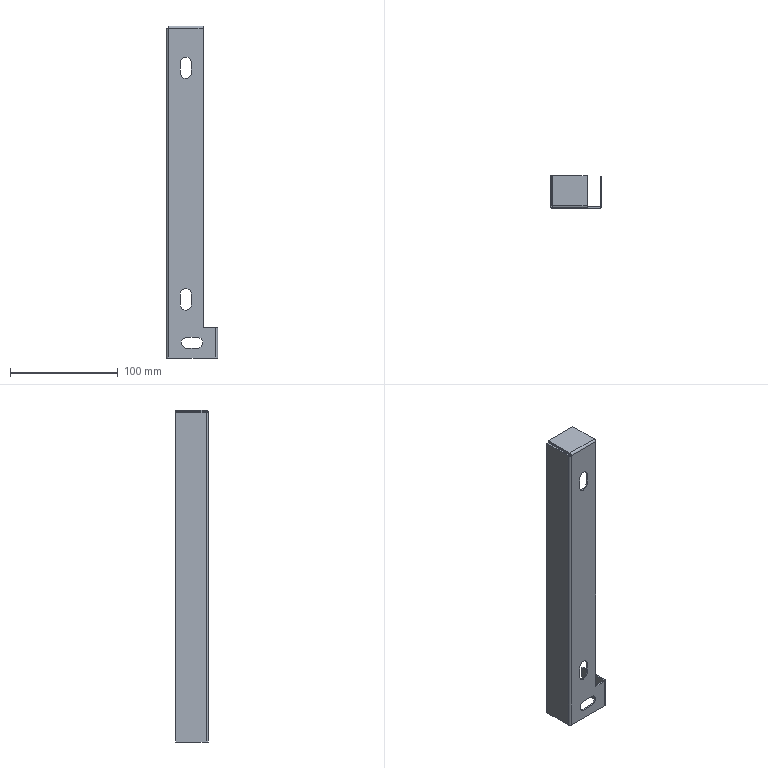Part | SolidWorks | features ICE 4, EdgeFlange 3, FlatPattern 1, SMBaseFlange 1, SheetMetal 1 | 1 solid | 46 faces | box 47.5 x 30 x 307.5 mm | volume 30771 mm3 | plane 32 | cylinder 14 | commonest cylinder face diameters 10 x8 1 x3 4 x3
STEP:
#1=CARTESIAN_POINT('',(23.,0.,59.2));
#2=VERTEX_POINT('',#1);
#3=CARTESIAN_POINT('',(18.,0.,64.2));
#4=VERTEX_POINT('',#3);
#5=CARTESIAN_POINT('',(18.,0.,59.2));
#6=DIRECTION('',(0.,-1.,0.));
#7=DIRECTION('',(0.,0.,1.));
#8=AXIS2_PLACEMENT_3D('',#5,#6,#7);
#9=CIRCLE('',#8,5.);
#10=EDGE_CURVE('',#2,#4,#9,.T.);
#11=ORIENTED_EDGE('',*,*,#10,.T.);
#12=CARTESIAN_POINT('',(18.,1.5,64.2));
#13=VERTEX_POINT('',#12);
#14=CARTESIAN_POINT('',(18.,-0.001,64.2));
#15=DIRECTION('',(0.,1.,0.));
#16=VECTOR('',#15,1000.);
#17=LINE('',#14,#16);
#18=EDGE_CURVE('',#4,#13,#17,.T.);
#19=ORIENTED_EDGE('',*,*,#18,.T.);
#20=CARTESIAN_POINT('',(23.,1.5,59.2));
#21=VERTEX_POINT('',#20);
#22=CARTESIAN_POINT('',(18.,1.5,59.2));
#23=DIRECTION('',(0.,1.,0.));
#24=DIRECTION('',(0.,0.,1.));
#25=AXIS2_PLACEMENT_3D('',#22,#23,#24);
#26=CIRCLE('',#25,5.);
#27=EDGE_CURVE('',#13,#21,#26,.T.);
#28=ORIENTED_EDGE('',*,*,#27,.T.);
#29=CARTESIAN_POINT('',(23.,-0.001,59.2));
#30=DIRECTION('',(0.,1.,0.));
#31=VECTOR('',#30,1000.);
#32=LINE('',#29,#31);
#33=EDGE_CURVE('',#2,#21,#32,.T.);
#34=ORIENTED_EDGE('',*,*,#33,.F.);
#35=EDGE_LOOP('',(#11,#19,#28,#34));
#36=FACE_OUTER_BOUND('',#35,.T.);
#37=CARTESIAN_POINT('',(18.,-0.001,59.2));
#38=DIRECTION('',(0.,1.,0.));
#39=DIRECTION('',(0.,0.,1.));
#40=AXIS2_PLACEMENT_3D('',#37,#38,#39);
#41=CYLINDRICAL_SURFACE('',#40,5.);
#42=ADVANCED_FACE('',(#36),#41,.F.);
#43=CARTESIAN_POINT('',(18.,0.,278.7));
#44=VERTEX_POINT('',#43);
#45=CARTESIAN_POINT('',(23.,0.,273.7));
#46=VERTEX_POINT('',#45);
#47=CARTESIAN_POINT('',(18.,0.,273.7));
#48=DIRECTION('',(0.,1.,0.));
#49=DIRECTION('',(0.,0.,1.));
#50=AXIS2_PLACEMENT_3D('',#47,#48,#49);
#51=CIRCLE('',#50,5.);
#52=EDGE_CURVE('',#44,#46,#51,.T.);
#53=ORIENTED_EDGE('',*,*,#52,.F.);
#54=CARTESIAN_POINT('',(18.,1.5,278.7));
#55=VERTEX_POINT('',#54);
#56=CARTESIAN_POINT('',(18.,-8.5,278.7));
#57=DIRECTION('',(0.,1.,0.));
#58=VECTOR('',#57,1000.);
#59=LINE('',#56,#58);
#60=EDGE_CURVE('',#44,#55,#59,.T.);
#61=ORIENTED_EDGE('',*,*,#60,.T.);
#62=CARTESIAN_POINT('',(23.,1.5,273.7));
#63=VERTEX_POINT('',#62);
#64=CARTESIAN_POINT('',(18.,1.5,273.7));
#65=DIRECTION('',(0.,1.,0.));
#66=DIRECTION('',(0.,0.,1.));
#67=AXIS2_PLACEMENT_3D('',#64,#65,#66);
#68=CIRCLE('',#67,5.);
#69=EDGE_CURVE('',#55,#63,#68,.T.);
#70=ORIENTED_EDGE('',*,*,#69,.T.);
#71=CARTESIAN_POINT('',(23.,-8.5,273.7));
#72=DIRECTION('',(0.,1.,0.));
#73=VECTOR('',#72,1000.);
#74=LINE('',#71,#73);
#75=EDGE_CURVE('',#46,#63,#74,.T.);
#76=ORIENTED_EDGE('',*,*,#75,.F.);
#77=EDGE_LOOP('',(#53,#61,#70,#76));
#78=FACE_OUTER_BOUND('',#77,.T.);
#79=CARTESIAN_POINT('',(18.,-8.5,273.7));
#80=DIRECTION('',(0.,1.,0.));
#81=DIRECTION('',(0.,0.,1.));
#82=AXIS2_PLACEMENT_3D('',#79,#80,#81);
#83=CYLINDRICAL_SURFACE('',#82,5.);
#84=ADVANCED_FACE('',(#78),#83,.F.);
#85=CARTESIAN_POINT('',(34.,1.5,28.));
#86=VERTEX_POINT('',#85);
#87=CARTESIAN_POINT('',(34.,1.5,305.5));
#88=VERTEX_POINT('',#87);
#89=CARTESIAN_POINT('',(34.,1.5,305.5));
#90=DIRECTION('',(0.,0.,1.));
#91=VECTOR('',#90,1000.);
#92=LINE('',#89,#91);
#93=EDGE_CURVE('',#86,#88,#92,.T.);
#94=ORIENTED_EDGE('',*,*,#93,.T.);
#95=CARTESIAN_POINT('',(34.,0.,305.5));
#96=VERTEX_POINT('',#95);
#97=CARTESIAN_POINT('',(34.,1.5,305.5));
#98=DIRECTION('',(0.,-1.,0.));
#99=VECTOR('',#98,1000.);
#100=LINE('',#97,#99);
#101=EDGE_CURVE('',#88,#96,#100,.T.);
#102=ORIENTED_EDGE('',*,*,#101,.T.);
#103=CARTESIAN_POINT('',(34.,0.,28.));
#104=VERTEX_POINT('',#103);
#105=CARTESIAN_POINT('',(34.,0.,307.5));
#106=DIRECTION('',(0.,0.,1.));
#107=VECTOR('',#106,1000.);
#108=LINE('',#105,#107);
#109=EDGE_CURVE('',#104,#96,#108,.T.);
#110=ORIENTED_EDGE('',*,*,#109,.F.);
#111=CARTESIAN_POINT('',(34.,0.,28.));
#112=DIRECTION('',(0.,1.,0.));
#113=VECTOR('',#112,1000.);
#114=LINE('',#111,#113);
#115=EDGE_CURVE('',#104,#86,#114,.T.);
#116=ORIENTED_EDGE('',*,*,#115,.T.);
#117=EDGE_LOOP('',(#94,#102,#110,#116));
#118=FACE_OUTER_BOUND('',#117,.T.);
#119=CARTESIAN_POINT('',(34.,0.,307.5));
#120=DIRECTION('',(-1.,0.,0.));
#121=DIRECTION('',(0.,0.,1.));
#122=AXIS2_PLACEMENT_3D('',#119,#120,#121);
#123=PLANE('',#122);
#124=ADVANCED_FACE('',(#118),#123,.F.);
#125=CARTESIAN_POINT('',(34.,2.,307.5));
#126=VERTEX_POINT('',#125);
#127=CARTESIAN_POINT('',(34.,30.,307.5));
#128=VERTEX_POINT('',#127);
#129=CARTESIAN_POINT('',(34.,0.,307.5));
#130=DIRECTION('',(0.,1.,0.));
#131=VECTOR('',#130,1000.);
#132=LINE('',#129,#131);
#133=EDGE_CURVE('',#126,#128,#132,.T.);
#134=ORIENTED_EDGE('',*,*,#133,.F.);
#135=CARTESIAN_POINT('',(34.,2.,306.));
#136=VERTEX_POINT('',#135);
#137=CARTESIAN_POINT('',(34.,2.,307.5));
#138=DIRECTION('',(0.,0.,-1.));
#139=VECTOR('',#138,1000.);
#140=LINE('',#137,#139);
#141=EDGE_CURVE('',#126,#136,#140,.T.);
#142=ORIENTED_EDGE('',*,*,#141,.T.);
#143=CARTESIAN_POINT('',(34.,30.,306.));
#144=VERTEX_POINT('',#143);
#145=CARTESIAN_POINT('',(34.,0.,306.));
#146=DIRECTION('',(0.,1.,0.));
#147=VECTOR('',#146,1000.);
#148=LINE('',#145,#147);
#149=EDGE_CURVE('',#136,#144,#148,.T.);
#150=ORIENTED_EDGE('',*,*,#149,.T.);
#151=CARTESIAN_POINT('',(34.,30.,307.5));
#152=DIRECTION('',(0.,0.,-1.));
#153=VECTOR('',#152,1000.);
#154=LINE('',#151,#153);
#155=EDGE_CURVE('',#128,#144,#154,.T.);
#156=ORIENTED_EDGE('',*,*,#155,.F.);
#157=EDGE_LOOP('',(#134,#142,#150,#156));
#158=FACE_OUTER_BOUND('',#157,.T.);
#159=CARTESIAN_POINT('',(34.,0.,307.5));
#160=DIRECTION('',(-1.,0.,0.));
#161=DIRECTION('',(0.,0.,1.));
#162=AXIS2_PLACEMENT_3D('',#159,#160,#161);
#163=PLANE('',#162);
#164=ADVANCED_FACE('',(#158),#163,.F.);
#165=CARTESIAN_POINT('',(0.,2.,305.5));
#166=VERTEX_POINT('',#165);
#167=CARTESIAN_POINT('',(1.5,2.,305.5));
#168=VERTEX_POINT('',#167);
#169=CARTESIAN_POINT('',(0.,2.,305.5));
#170=DIRECTION('',(1.,0.,0.));
#171=VECTOR('',#170,1000.);
#172=LINE('',#169,#171);
#173=EDGE_CURVE('',#166,#168,#172,.T.);
#174=ORIENTED_EDGE('',*,*,#173,.F.);
#175=CARTESIAN_POINT('',(2.,0.,305.5));
#176=VERTEX_POINT('',#175);
#177=CARTESIAN_POINT('',(2.,2.,305.5));
#178=DIRECTION('',(0.,0.,1.));
#179=DIRECTION('',(-1.,0.,0.));
#180=AXIS2_PLACEMENT_3D('',#177,#178,#179);
#181=CIRCLE('',#180,2.);
#182=EDGE_CURVE('',#166,#176,#181,.T.);
#183=ORIENTED_EDGE('',*,*,#182,.T.);
#184=CARTESIAN_POINT('',(2.,1.5,305.5));
#185=VERTEX_POINT('',#184);
#186=CARTESIAN_POINT('',(2.,1.5,305.5));
#187=DIRECTION('',(0.,-1.,0.));
#188=VECTOR('',#187,1000.);
#189=LINE('',#186,#188);
#190=EDGE_CURVE('',#185,#176,#189,.T.);
#191=ORIENTED_EDGE('',*,*,#190,.F.);
#192=CARTESIAN_POINT('',(2.,2.,305.5));
#193=DIRECTION('',(0.,0.,1.));
#194=DIRECTION('',(1.,0.,0.));
#195=AXIS2_PLACEMENT_3D('',#192,#193,#194);
#196=CIRCLE('',#195,0.5);
#197=EDGE_CURVE('',#168,#185,#196,.T.);
#198=ORIENTED_EDGE('',*,*,#197,.F.);
#199=EDGE_LOOP('',(#174,#183,#191,#198));
#200=FACE_OUTER_BOUND('',#199,.T.);
#201=CARTESIAN_POINT('',(0.,2.,305.5));
#202=DIRECTION('',(0.,0.,1.));
#203=DIRECTION('',(1.,0.,0.));
#204=AXIS2_PLACEMENT_3D('',#201,#202,#203);
#205=PLANE('',#204);
#206=ADVANCED_FACE('',(#200),#205,.T.);
#207=CARTESIAN_POINT('',(0.,30.,305.5));
#208=VERTEX_POINT('',#207);
#209=CARTESIAN_POINT('',(0.,30.,305.5));
#210=DIRECTION('',(0.,-1.,0.));
#211=VECTOR('',#210,1000.);
#212=LINE('',#209,#211);
#213=EDGE_CURVE('',#208,#166,#212,.T.);
#214=ORIENTED_EDGE('',*,*,#213,.T.);
#215=ORIENTED_EDGE('',*,*,#173,.T.);
#216=CARTESIAN_POINT('',(1.5,30.,305.5));
#217=VERTEX_POINT('',#216);
#218=CARTESIAN_POINT('',(1.5,30.,305.5));
#219=DIRECTION('',(0.,-1.,0.));
#220=VECTOR('',#219,1000.);
#221=LINE('',#218,#220);
#222=EDGE_CURVE('',#217,#168,#221,.T.);
#223=ORIENTED_EDGE('',*,*,#222,.F.);
#224=CARTESIAN_POINT('',(0.,30.,305.5));
#225=DIRECTION('',(1.,0.,0.));
#226=VECTOR('',#225,1000.);
#227=LINE('',#224,#226);
#228=EDGE_CURVE('',#208,#217,#227,.T.);
#229=ORIENTED_EDGE('',*,*,#228,.F.);
#230=EDGE_LOOP('',(#214,#215,#223,#229));
#231=FACE_OUTER_BOUND('',#230,.T.);
#232=CARTESIAN_POINT('',(2.,1.5,305.5));
#233=DIRECTION('',(0.,0.,1.));
#234=DIRECTION('',(1.,0.,0.));
#235=AXIS2_PLACEMENT_3D('',#232,#233,#234);
#236=PLANE('',#235);
#237=ADVANCED_FACE('',(#231),#236,.T.);
#238=CARTESIAN_POINT('',(2.,0.,0.));
#239=VERTEX_POINT('',#238);
#240=CARTESIAN_POINT('',(2.,1.5,0.));
#241=VERTEX_POINT('',#240);
#242=CARTESIAN_POINT('',(2.,0.,0.));
#243=DIRECTION('',(0.,1.,0.));
#244=VECTOR('',#243,1000.);
#245=LINE('',#242,#244);
#246=EDGE_CURVE('',#239,#241,#245,.T.);
#247=ORIENTED_EDGE('',*,*,#246,.F.);
#248=CARTESIAN_POINT('',(0.,2.,0.));
#249=VERTEX_POINT('',#248);
#250=CARTESIAN_POINT('',(2.,2.,0.));
#251=DIRECTION('',(0.,0.,1.));
#252=DIRECTION('',(-1.,0.,0.));
#253=AXIS2_PLACEMENT_3D('',#250,#251,#252);
#254=CIRCLE('',#253,2.);
#255=EDGE_CURVE('',#249,#239,#254,.T.);
#256=ORIENTED_EDGE('',*,*,#255,.F.);
#257=CARTESIAN_POINT('',(1.5,2.,0.));
#258=VERTEX_POINT('',#257);
#259=CARTESIAN_POINT('',(1.5,2.,0.));
#260=DIRECTION('',(-1.,0.,0.));
#261=VECTOR('',#260,1000.);
#262=LINE('',#259,#261);
#263=EDGE_CURVE('',#258,#249,#262,.T.);
#264=ORIENTED_EDGE('',*,*,#263,.F.);
#265=CARTESIAN_POINT('',(2.,2.,0.));
#266=DIRECTION('',(0.,0.,1.));
#267=DIRECTION('',(1.,0.,0.));
#268=AXIS2_PLACEMENT_3D('',#265,#266,#267);
#269=CIRCLE('',#268,0.5);
#270=EDGE_CURVE('',#258,#241,#269,.T.);
#271=ORIENTED_EDGE('',*,*,#270,.T.);
#272=EDGE_LOOP('',(#247,#256,#264,#271));
#273=FACE_OUTER_BOUND('',#272,.T.);
#274=CARTESIAN_POINT('',(2.,0.,0.));
#275=DIRECTION('',(0.,0.,-1.));
#276=DIRECTION('',(-1.,0.,0.));
#277=AXIS2_PLACEMENT_3D('',#274,#275,#276);
#278=PLANE('',#277);
#279=ADVANCED_FACE('',(#273),#278,.T.);
#280=CARTESIAN_POINT('',(13.,0.,59.2));
#281=VERTEX_POINT('',#280);
#282=CARTESIAN_POINT('',(13.,0.,49.2));
#283=VERTEX_POINT('',#282);
#284=CARTESIAN_POINT('',(13.,0.,59.2));
#285=DIRECTION('',(0.,0.,-1.));
#286=VECTOR('',#285,1000.);
#287=LINE('',#284,#286);
#288=EDGE_CURVE('',#281,#283,#287,.T.);
#289=ORIENTED_EDGE('',*,*,#288,.F.);
#290=CARTESIAN_POINT('',(18.,0.,59.2));
#291=DIRECTION('',(0.,-1.,0.));
#292=DIRECTION('',(0.,0.,1.));
#293=AXIS2_PLACEMENT_3D('',#290,#291,#292);
#294=CIRCLE('',#293,5.);
#295=EDGE_CURVE('',#4,#281,#294,.T.);
#296=ORIENTED_EDGE('',*,*,#295,.F.);
#297=ORIENTED_EDGE('',*,*,#10,.F.);
#298=CARTESIAN_POINT('',(23.,0.,49.2));
#299=VERTEX_POINT('',#298);
#300=CARTESIAN_POINT('',(23.,0.,59.2));
#301=DIRECTION('',(0.,0.,1.));
#302=VECTOR('',#301,1000.);
#303=LINE('',#300,#302);
#304=EDGE_CURVE('',#299,#2,#303,.T.);
#305=ORIENTED_EDGE('',*,*,#304,.F.);
#306=CARTESIAN_POINT('',(18.,0.,49.2));
#307=DIRECTION('',(0.,-1.,0.));
#308=DIRECTION('',(0.,0.,1.));
#309=AXIS2_PLACEMENT_3D('',#306,#307,#308);
#310=CIRCLE('',#309,5.);
#311=EDGE_CURVE('',#283,#299,#310,.T.);
#312=ORIENTED_EDGE('',*,*,#311,.F.);
#313=EDGE_LOOP('',(#289,#296,#297,#305,#312));
#314=FACE_BOUND('',#313,.T.);
#315=CARTESIAN_POINT('',(13.,0.,263.7));
#316=VERTEX_POINT('',#315);
#317=CARTESIAN_POINT('',(13.,0.,273.7));
#318=VERTEX_POINT('',#317);
#319=CARTESIAN_POINT('',(13.,0.,305.5));
#320=DIRECTION('',(0.,0.,1.));
#321=VECTOR('',#320,1000.);
#322=LINE('',#319,#321);
#323=EDGE_CURVE('',#316,#318,#322,.T.);
#324=ORIENTED_EDGE('',*,*,#323,.T.);
#325=CARTESIAN_POINT('',(18.,0.,273.7));
#326=DIRECTION('',(0.,1.,0.));
#327=DIRECTION('',(0.,0.,1.));
#328=AXIS2_PLACEMENT_3D('',#325,#326,#327);
#329=CIRCLE('',#328,5.);
#330=EDGE_CURVE('',#318,#44,#329,.T.);
#331=ORIENTED_EDGE('',*,*,#330,.T.);
#332=ORIENTED_EDGE('',*,*,#52,.T.);
#333=CARTESIAN_POINT('',(23.,0.,263.7));
#334=VERTEX_POINT('',#333);
#335=CARTESIAN_POINT('',(23.,0.,305.5));
#336=DIRECTION('',(0.,0.,-1.));
#337=VECTOR('',#336,1000.);
#338=LINE('',#335,#337);
#339=EDGE_CURVE('',#46,#334,#338,.T.);
#340=ORIENTED_EDGE('',*,*,#339,.T.);
#341=CARTESIAN_POINT('',(18.,0.,263.7));
#342=DIRECTION('',(0.,1.,0.));
#343=DIRECTION('',(0.,0.,1.));
#344=AXIS2_PLACEMENT_3D('',#341,#342,#343);
#345=CIRCLE('',#344,5.);
#346=EDGE_CURVE('',#334,#316,#345,.T.);
#347=ORIENTED_EDGE('',*,*,#346,.T.);
#348=EDGE_LOOP('',(#324,#331,#332,#340,#347));
#349=FACE_BOUND('',#348,.T.);
#350=CARTESIAN_POINT('',(28.8,0.,9.));
#351=VERTEX_POINT('',#350);
#352=CARTESIAN_POINT('',(18.8,0.,9.));
#353=VERTEX_POINT('',#352);
#354=CARTESIAN_POINT('',(0.,0.,9.));
#355=DIRECTION('',(-1.,0.,0.));
#356=VECTOR('',#355,1000.);
#357=LINE('',#354,#356);
#358=EDGE_CURVE('',#351,#353,#357,.T.);
#359=ORIENTED_EDGE('',*,*,#358,.T.);
#360=CARTESIAN_POINT('',(18.8,0.,19.));
#361=VERTEX_POINT('',#360);
#362=CARTESIAN_POINT('',(18.8,0.,14.));
#363=DIRECTION('',(0.,1.,0.));
#364=DIRECTION('',(0.,0.,1.));
#365=AXIS2_PLACEMENT_3D('',#362,#363,#364);
#366=CIRCLE('',#365,5.);
#367=EDGE_CURVE('',#353,#361,#366,.T.);
#368=ORIENTED_EDGE('',*,*,#367,.T.);
#369=CARTESIAN_POINT('',(28.8,0.,19.));
#370=VERTEX_POINT('',#369);
#371=CARTESIAN_POINT('',(0.,0.,19.));
#372=DIRECTION('',(1.,0.,0.));
#373=VECTOR('',#372,1000.);
#374=LINE('',#371,#373);
#375=EDGE_CURVE('',#361,#370,#374,.T.);
#376=ORIENTED_EDGE('',*,*,#375,.T.);
#377=CARTESIAN_POINT('',(28.8,0.,14.));
#378=DIRECTION('',(0.,1.,0.));
#379=DIRECTION('',(0.,0.,1.));
#380=AXIS2_PLACEMENT_3D('',#377,#378,#379);
#381=CIRCLE('',#380,5.);
#382=EDGE_CURVE('',#370,#351,#381,.T.);
#383=ORIENTED_EDGE('',*,*,#382,.T.);
#384=EDGE_LOOP('',(#359,#368,#376,#383));
#385=FACE_BOUND('',#384,.T.);
#386=CARTESIAN_POINT('',(45.5,0.,28.));
#387=VERTEX_POINT('',#386);
#388=CARTESIAN_POINT('',(45.5,0.,28.));
#389=DIRECTION('',(-1.,0.,0.));
#390=VECTOR('',#389,1000.);
#391=LINE('',#388,#390);
#392=EDGE_CURVE('',#387,#104,#391,.T.);
#393=ORIENTED_EDGE('',*,*,#392,.T.);
#394=ORIENTED_EDGE('',*,*,#109,.T.);
#395=CARTESIAN_POINT('',(0.,0.,305.5));
#396=DIRECTION('',(1.,0.,0.));
#397=VECTOR('',#396,1000.);
#398=LINE('',#395,#397);
#399=EDGE_CURVE('',#176,#96,#398,.T.);
#400=ORIENTED_EDGE('',*,*,#399,.F.);
#401=CARTESIAN_POINT('',(2.,0.,305.5));
#402=DIRECTION('',(0.,0.,-1.));
#403=VECTOR('',#402,1000.);
#404=LINE('',#401,#403);
#405=EDGE_CURVE('',#176,#239,#404,.T.);
#406=ORIENTED_EDGE('',*,*,#405,.T.);
#407=CARTESIAN_POINT('',(45.5,0.,0.));
#408=VERTEX_POINT('',#407);
#409=CARTESIAN_POINT('',(0.,0.,0.));
#410=DIRECTION('',(1.,0.,0.));
#411=VECTOR('',#410,1000.);
#412=LINE('',#409,#411);
#413=EDGE_CURVE('',#239,#408,#412,.T.);
#414=ORIENTED_EDGE('',*,*,#413,.T.);
#415=CARTESIAN_POINT('',(45.5,0.,305.5));
#416=DIRECTION('',(0.,0.,-1.));
#417=VECTOR('',#416,1000.);
#418=LINE('',#415,#417);
#419=EDGE_CURVE('',#387,#408,#418,.T.);
#420=ORIENTED_EDGE('',*,*,#419,.F.);
#421=EDGE_LOOP('',(#393,#394,#400,#406,#414,#420));
#422=FACE_OUTER_BOUND('',#421,.T.);
#423=CARTESIAN_POINT('',(0.,0.,305.5));
#424=DIRECTION('',(0.,1.,0.));
#425=DIRECTION('',(0.,0.,1.));
#426=AXIS2_PLACEMENT_3D('',#423,#424,#425);
#427=PLANE('',#426);
#428=ADVANCED_FACE('',(#314,#349,#385,#422),#427,.F.);
#429=CARTESIAN_POINT('',(13.,1.5,59.2));
#430=VERTEX_POINT('',#429);
#431=CARTESIAN_POINT('',(18.,1.5,59.2));
#432=DIRECTION('',(0.,1.,0.));
#433=DIRECTION('',(0.,0.,1.));
#434=AXIS2_PLACEMENT_3D('',#431,#432,#433);
#435=CIRCLE('',#434,5.);
#436=EDGE_CURVE('',#430,#13,#435,.T.);
#437=ORIENTED_EDGE('',*,*,#436,.F.);
#438=CARTESIAN_POINT('',(13.,1.5,49.2));
#439=VERTEX_POINT('',#438);
#440=CARTESIAN_POINT('',(13.,1.5,59.2));
#441=DIRECTION('',(0.,0.,1.));
#442=VECTOR('',#441,1000.);
#443=LINE('',#440,#442);
#444=EDGE_CURVE('',#439,#430,#443,.T.);
#445=ORIENTED_EDGE('',*,*,#444,.F.);
#446=CARTESIAN_POINT('',(23.,1.5,49.2));
#447=VERTEX_POINT('',#446);
#448=CARTESIAN_POINT('',(18.,1.5,49.2));
#449=DIRECTION('',(0.,1.,0.));
#450=DIRECTION('',(0.,0.,1.));
#451=AXIS2_PLACEMENT_3D('',#448,#449,#450);
#452=CIRCLE('',#451,5.);
#453=EDGE_CURVE('',#447,#439,#452,.T.);
#454=ORIENTED_EDGE('',*,*,#453,.F.);
#455=CARTESIAN_POINT('',(23.,1.5,59.2));
#456=DIRECTION('',(0.,0.,-1.));
#457=VECTOR('',#456,1000.);
#458=LINE('',#455,#457);
#459=EDGE_CURVE('',#21,#447,#458,.T.);
#460=ORIENTED_EDGE('',*,*,#459,.F.);
#461=ORIENTED_EDGE('',*,*,#27,.F.);
#462=EDGE_LOOP('',(#437,#445,#454,#460,#461));
#463=FACE_BOUND('',#462,.T.);
#464=CARTESIAN_POINT('',(13.,1.5,273.7));
#465=VERTEX_POINT('',#464);
#466=CARTESIAN_POINT('',(18.,1.5,273.7));
#467=DIRECTION('',(0.,1.,0.));
#468=DIRECTION('',(0.,0.,1.));
#469=AXIS2_PLACEMENT_3D('',#466,#467,#468);
#470=CIRCLE('',#469,5.);
#471=EDGE_CURVE('',#465,#55,#470,.T.);
#472=ORIENTED_EDGE('',*,*,#471,.F.);
#473=CARTESIAN_POINT('',(13.,1.5,263.7));
#474=VERTEX_POINT('',#473);
#475=CARTESIAN_POINT('',(13.,1.5,273.7));
#476=DIRECTION('',(0.,0.,1.));
#477=VECTOR('',#476,1000.);
#478=LINE('',#475,#477);
#479=EDGE_CURVE('',#474,#465,#478,.T.);
#480=ORIENTED_EDGE('',*,*,#479,.F.);
#481=CARTESIAN_POINT('',(23.,1.5,263.7));
#482=VERTEX_POINT('',#481);
#483=CARTESIAN_POINT('',(18.,1.5,263.7));
#484=DIRECTION('',(0.,1.,0.));
#485=DIRECTION('',(0.,0.,1.));
#486=AXIS2_PLACEMENT_3D('',#483,#484,#485);
#487=CIRCLE('',#486,5.);
#488=EDGE_CURVE('',#482,#474,#487,.T.);
#489=ORIENTED_EDGE('',*,*,#488,.F.);
#490=CARTESIAN_POINT('',(23.,1.5,273.7));
#491=DIRECTION('',(0.,0.,-1.));
#492=VECTOR('',#491,1000.);
#493=LINE('',#490,#492);
#494=EDGE_CURVE('',#63,#482,#493,.T.);
#495=ORIENTED_EDGE('',*,*,#494,.F.);
#496=ORIENTED_EDGE('',*,*,#69,.F.);
#497=EDGE_LOOP('',(#472,#480,#489,#495,#496));
#498=FACE_BOUND('',#497,.T.);
#499=CARTESIAN_POINT('',(18.8,1.5,9.));
#500=VERTEX_POINT('',#499);
#501=CARTESIAN_POINT('',(18.8,1.5,19.));
#502=VERTEX_POINT('',#501);
#503=CARTESIAN_POINT('',(18.8,1.5,14.));
#504=DIRECTION('',(0.,1.,0.));
#505=DIRECTION('',(0.,0.,1.));
#506=AXIS2_PLACEMENT_3D('',#503,#504,#505);
#507=CIRCLE('',#506,5.);
#508=EDGE_CURVE('',#500,#502,#507,.T.);
#509=ORIENTED_EDGE('',*,*,#508,.F.);
#510=CARTESIAN_POINT('',(28.8,1.5,9.));
#511=VERTEX_POINT('',#510);
#512=CARTESIAN_POINT('',(18.8,1.5,9.));
#513=DIRECTION('',(-1.,0.,0.));
#514=VECTOR('',#513,1000.);
#515=LINE('',#512,#514);
#516=EDGE_CURVE('',#511,#500,#515,.T.);
#517=ORIENTED_EDGE('',*,*,#516,.F.);
#518=CARTESIAN_POINT('',(28.8,1.5,19.));
#519=VERTEX_POINT('',#518);
#520=CARTESIAN_POINT('',(28.8,1.5,14.));
#521=DIRECTION('',(0.,1.,0.));
#522=DIRECTION('',(0.,0.,1.));
#523=AXIS2_PLACEMENT_3D('',#520,#521,#522);
#524=CIRCLE('',#523,5.);
#525=EDGE_CURVE('',#519,#511,#524,.T.);
#526=ORIENTED_EDGE('',*,*,#525,.F.);
#527=CARTESIAN_POINT('',(18.8,1.5,19.));
#528=DIRECTION('',(1.,0.,0.));
#529=VECTOR('',#528,1000.);
#530=LINE('',#527,#529);
#531=EDGE_CURVE('',#502,#519,#530,.T.);
#532=ORIENTED_EDGE('',*,*,#531,.F.);
#533=EDGE_LOOP('',(#509,#517,#526,#532));
#534=FACE_BOUND('',#533,.T.);
#535=ORIENTED_EDGE('',*,*,#93,.F.);
#536=CARTESIAN_POINT('',(45.5,1.5,28.));
#537=VERTEX_POINT('',#536);
#538=CARTESIAN_POINT('',(0.,1.5,28.));
#539=DIRECTION('',(-1.,0.,0.));
#540=VECTOR('',#539,1000.);
#541=LINE('',#538,#540);
#542=EDGE_CURVE('',#537,#86,#541,.T.);
#543=ORIENTED_EDGE('',*,*,#542,.F.);
#544=CARTESIAN_POINT('',(45.5,1.5,0.));
#545=VERTEX_POINT('',#544);
#546=CARTESIAN_POINT('',(45.5,1.5,305.5));
#547=DIRECTION('',(0.,0.,-1.));
#548=VECTOR('',#547,1000.);
#549=LINE('',#546,#548);
#550=EDGE_CURVE('',#537,#545,#549,.T.);
#551=ORIENTED_EDGE('',*,*,#550,.T.);
#552=CARTESIAN_POINT('',(0.,1.5,0.));
#553=DIRECTION('',(1.,0.,0.));
#554=VECTOR('',#553,1000.);
#555=LINE('',#552,#554);
#556=EDGE_CURVE('',#241,#545,#555,.T.);
#557=ORIENTED_EDGE('',*,*,#556,.F.);
#558=CARTESIAN_POINT('',(2.,1.5,305.5));
#559=DIRECTION('',(0.,0.,-1.));
#560=VECTOR('',#559,1000.);
#561=LINE('',#558,#560);
#562=EDGE_CURVE('',#185,#241,#561,.T.);
#563=ORIENTED_EDGE('',*,*,#562,.F.);
#564=CARTESIAN_POINT('',(0.,1.5,305.5));
#565=DIRECTION('',(1.,0.,0.));
#566=VECTOR('',#565,1000.);
#567=LINE('',#564,#566);
#568=EDGE_CURVE('',#185,#88,#567,.T.);
#569=ORIENTED_EDGE('',*,*,#568,.T.);
#570=EDGE_LOOP('',(#535,#543,#551,#557,#563,#569));
#571=FACE_OUTER_BOUND('',#570,.T.);
#572=CARTESIAN_POINT('',(0.,1.5,305.5));
#573=DIRECTION('',(0.,1.,0.));
#574=DIRECTION('',(0.,0.,1.));
#575=AXIS2_PLACEMENT_3D('',#572,#573,#574);
#576=PLANE('',#575);
#577=ADVANCED_FACE('',(#463,#498,#534,#571),#576,.T.);
#578=ORIENTED_EDGE('',*,*,#270,.F.);
#579=CARTESIAN_POINT('',(1.5,2.,305.5));
#580=DIRECTION('',(0.,0.,-1.));
#581=VECTOR('',#580,1000.);
#582=LINE('',#579,#581);
#583=EDGE_CURVE('',#168,#258,#582,.T.);
#584=ORIENTED_EDGE('',*,*,#583,.F.);
#585=ORIENTED_EDGE('',*,*,#197,.T.);
#586=ORIENTED_EDGE('',*,*,#562,.T.);
#587=EDGE_LOOP('',(#578,#584,#585,#586));
#588=FACE_OUTER_BOUND('',#587,.T.);
#589=CARTESIAN_POINT('',(2.,2.,305.5));
#590=DIRECTION('',(0.,0.,-1.));
#591=DIRECTION('',(-1.,0.,0.));
#592=AXIS2_PLACEMENT_3D('',#589,#590,#591);
#593=CYLINDRICAL_SURFACE('',#592,0.5);
#594=ADVANCED_FACE('',(#588),#593,.F.);
#595=CARTESIAN_POINT('',(1.5,30.,0.));
#596=VERTEX_POINT('',#595);
#597=CARTESIAN_POINT('',(1.5,30.,0.));
#598=DIRECTION('',(0.,-1.,0.));
#599=VECTOR('',#598,1000.);
#600=LINE('',#597,#599);
#601=EDGE_CURVE('',#596,#258,#600,.T.);
#602=ORIENTED_EDGE('',*,*,#601,.F.);
#603=CARTESIAN_POINT('',(1.5,30.,305.5));
#604=DIRECTION('',(0.,0.,-1.));
#605=VECTOR('',#604,1000.);
#606=LINE('',#603,#605);
#607=EDGE_CURVE('',#217,#596,#606,.T.);
#608=ORIENTED_EDGE('',*,*,#607,.F.);
#609=ORIENTED_EDGE('',*,*,#222,.T.);
#610=ORIENTED_EDGE('',*,*,#583,.T.);
#611=EDGE_LOOP('',(#602,#608,#609,#610));
#612=FACE_OUTER_BOUND('',#611,.T.);
#613=CARTESIAN_POINT('',(1.5,30.,305.5));
#614=DIRECTION('',(1.,0.,0.));
#615=DIRECTION('',(0.,1.,0.));
#616=AXIS2_PLACEMENT_3D('',#613,#614,#615);
#617=PLANE('',#616);
#618=ADVANCED_FACE('',(#612),#617,.T.);
#619=CARTESIAN_POINT('',(0.,30.,0.));
#620=VERTEX_POINT('',#619);
#621=CARTESIAN_POINT('',(0.,30.,0.));
#622=DIRECTION('',(1.,0.,0.));
#623=VECTOR('',#622,1000.);
#624=LINE('',#621,#623);
#625=EDGE_CURVE('',#620,#596,#624,.T.);
#626=ORIENTED_EDGE('',*,*,#625,.F.);
#627=CARTESIAN_POINT('',(0.,30.,305.5));
#628=DIRECTION('',(0.,0.,-1.));
#629=VECTOR('',#628,1000.);
#630=LINE('',#627,#629);
#631=EDGE_CURVE('',#208,#620,#630,.T.);
#632=ORIENTED_EDGE('',*,*,#631,.F.);
#633=ORIENTED_EDGE('',*,*,#228,.T.);
#634=ORIENTED_EDGE('',*,*,#607,.T.);
#635=EDGE_LOOP('',(#626,#632,#633,#634));
#636=FACE_OUTER_BOUND('',#635,.T.);
#637=CARTESIAN_POINT('',(0.,30.,305.5));
#638=DIRECTION('',(0.,1.,0.));
#639=DIRECTION('',(0.,0.,1.));
#640=AXIS2_PLACEMENT_3D('',#637,#638,#639);
#641=PLANE('',#640);
#642=ADVANCED_FACE('',(#636),#641,.T.);
#643=CARTESIAN_POINT('',(0.,30.,0.));
#644=DIRECTION('',(0.,-1.,0.));
#645=VECTOR('',#644,1000.);
#646=LINE('',#643,#645);
#647=EDGE_CURVE('',#620,#249,#646,.T.);
#648=ORIENTED_EDGE('',*,*,#647,.T.);
#649=CARTESIAN_POINT('',(0.,2.,305.5));
#650=DIRECTION('',(0.,0.,-1.));
#651=VECTOR('',#650,1000.);
#652=LINE('',#649,#651);
#653=EDGE_CURVE('',#166,#249,#652,.T.);
#654=ORIENTED_EDGE('',*,*,#653,.F.);
#655=ORIENTED_EDGE('',*,*,#213,.F.);
#656=ORIENTED_EDGE('',*,*,#631,.T.);
#657=EDGE_LOOP('',(#648,#654,#655,#656));
#658=FACE_OUTER_BOUND('',#657,.T.);
#659=CARTESIAN_POINT('',(0.,30.,305.5));
#660=DIRECTION('',(1.,0.,0.));
#661=DIRECTION('',(0.,1.,0.));
#662=AXIS2_PLACEMENT_3D('',#659,#660,#661);
#663=PLANE('',#662);
#664=ADVANCED_FACE('',(#658),#663,.F.);
#665=ORIENTED_EDGE('',*,*,#255,.T.);
#666=ORIENTED_EDGE('',*,*,#405,.F.);
#667=ORIENTED_EDGE('',*,*,#182,.F.);
#668=ORIENTED_EDGE('',*,*,#653,.T.);
#669=EDGE_LOOP('',(#665,#666,#667,#668));
#670=FACE_OUTER_BOUND('',#669,.T.);
#671=CARTESIAN_POINT('',(2.,2.,305.5));
#672=DIRECTION('',(0.,0.,-1.));
#673=DIRECTION('',(-1.,0.,0.));
#674=AXIS2_PLACEMENT_3D('',#671,#672,#673);
#675=CYLINDRICAL_SURFACE('',#674,2.);
#676=ADVANCED_FACE('',(#670),#675,.T.);
#677=ORIENTED_EDGE('',*,*,#601,.T.);
#678=ORIENTED_EDGE('',*,*,#263,.T.);
#679=ORIENTED_EDGE('',*,*,#647,.F.);
#680=ORIENTED_EDGE('',*,*,#625,.T.);
#681=EDGE_LOOP('',(#677,#678,#679,#680));
#682=FACE_OUTER_BOUND('',#681,.T.);
#683=CARTESIAN_POINT('',(2.,2.,0.));
#684=DIRECTION('',(0.,0.,1.));
#685=DIRECTION('',(1.,0.,0.));
#686=AXIS2_PLACEMENT_3D('',#683,#684,#685);
#687=PLANE('',#686);
#688=ADVANCED_FACE('',(#682),#687,.F.);
#689=CARTESIAN_POINT('',(2.,2.,306.));
#690=VERTEX_POINT('',#689);
#691=CARTESIAN_POINT('',(2.,2.,307.5));
#692=VERTEX_POINT('',#691);
#693=CARTESIAN_POINT('',(2.,2.,307.5));
#694=DIRECTION('',(0.,0.,1.));
#695=VECTOR('',#694,1000.);
#696=LINE('',#693,#695);
#697=EDGE_CURVE('',#690,#692,#696,.T.);
#698=ORIENTED_EDGE('',*,*,#697,.F.);
#699=CARTESIAN_POINT('',(2.,2.,305.5));
#700=DIRECTION('',(-1.,0.,0.));
#701=DIRECTION('',(0.,0.,-1.));
#702=AXIS2_PLACEMENT_3D('',#699,#700,#701);
#703=CIRCLE('',#702,0.5);
#704=EDGE_CURVE('',#185,#690,#703,.T.);
#705=ORIENTED_EDGE('',*,*,#704,.F.);
#706=ORIENTED_EDGE('',*,*,#190,.T.);
#707=CARTESIAN_POINT('',(2.,2.,305.5));
#708=DIRECTION('',(-1.,0.,0.));
#709=DIRECTION('',(0.,0.,-1.));
#710=AXIS2_PLACEMENT_3D('',#707,#708,#709);
#711=CIRCLE('',#710,2.);
#712=EDGE_CURVE('',#176,#692,#711,.T.);
#713=ORIENTED_EDGE('',*,*,#712,.T.);
#714=EDGE_LOOP('',(#698,#705,#706,#713));
#715=FACE_OUTER_BOUND('',#714,.T.);
#716=CARTESIAN_POINT('',(2.,2.,305.5));
#717=DIRECTION('',(-1.,0.,0.));
#718=DIRECTION('',(0.,0.,1.));
#719=AXIS2_PLACEMENT_3D('',#716,#717,#718);
#720=PLANE('',#719);
#721=ADVANCED_FACE('',(#715),#720,.T.);
#722=CARTESIAN_POINT('',(34.,2.,305.5));
#723=DIRECTION('',(1.,0.,0.));
#724=DIRECTION('',(0.,0.,1.));
#725=AXIS2_PLACEMENT_3D('',#722,#723,#724);
#726=CIRCLE('',#725,2.);
#727=EDGE_CURVE('',#126,#96,#726,.T.);
#728=ORIENTED_EDGE('',*,*,#727,.F.);
#729=CARTESIAN_POINT('',(2.,2.,307.5));
#730=DIRECTION('',(-1.,0.,0.));
#731=VECTOR('',#730,1000.);
#732=LINE('',#729,#731);
#733=EDGE_CURVE('',#126,#692,#732,.T.);
#734=ORIENTED_EDGE('',*,*,#733,.T.);
#735=ORIENTED_EDGE('',*,*,#712,.F.);
#736=ORIENTED_EDGE('',*,*,#399,.T.);
#737=EDGE_LOOP('',(#728,#734,#735,#736));
#738=FACE_OUTER_BOUND('',#737,.T.);
#739=CARTESIAN_POINT('',(45.5,2.,305.5));
#740=DIRECTION('',(1.,0.,0.));
#741=DIRECTION('',(0.,0.,1.));
#742=AXIS2_PLACEMENT_3D('',#739,#740,#741);
#743=CYLINDRICAL_SURFACE('',#742,2.);
#744=ADVANCED_FACE('',(#738),#743,.T.);
#745=CARTESIAN_POINT('',(2.,2.,306.));
#746=DIRECTION('',(1.,0.,0.));
#747=VECTOR('',#746,1000.);
#748=LINE('',#745,#747);
#749=EDGE_CURVE('',#690,#136,#748,.T.);
#750=ORIENTED_EDGE('',*,*,#749,.T.);
#751=CARTESIAN_POINT('',(34.,2.,305.5));
#752=DIRECTION('',(1.,0.,0.));
#753=DIRECTION('',(0.,0.,1.));
#754=AXIS2_PLACEMENT_3D('',#751,#752,#753);
#755=CIRCLE('',#754,0.5);
#756=EDGE_CURVE('',#136,#88,#755,.T.);
#757=ORIENTED_EDGE('',*,*,#756,.T.);
#758=ORIENTED_EDGE('',*,*,#568,.F.);
#759=ORIENTED_EDGE('',*,*,#704,.T.);
#760=EDGE_LOOP('',(#750,#757,#758,#759));
#761=FACE_OUTER_BOUND('',#760,.T.);
#762=CARTESIAN_POINT('',(45.5,2.,305.5));
#763=DIRECTION('',(1.,0.,0.));
#764=DIRECTION('',(0.,0.,1.));
#765=AXIS2_PLACEMENT_3D('',#762,#763,#764);
#766=CYLINDRICAL_SURFACE('',#765,0.5);
#767=ADVANCED_FACE('',(#761),#766,.F.);
#768=ORIENTED_EDGE('',*,*,#697,.T.);
#769=CARTESIAN_POINT('',(2.,30.,307.5));
#770=VERTEX_POINT('',#769);
#771=CARTESIAN_POINT('',(2.,0.,307.5));
#772=DIRECTION('',(0.,-1.,0.));
#773=VECTOR('',#772,1000.);
#774=LINE('',#771,#773);
#775=EDGE_CURVE('',#770,#692,#774,.T.);
#776=ORIENTED_EDGE('',*,*,#775,.F.);
#777=CARTESIAN_POINT('',(2.,30.,306.));
#778=VERTEX_POINT('',#777);
#779=CARTESIAN_POINT('',(2.,30.,307.5));
#780=DIRECTION('',(0.,0.,-1.));
#781=VECTOR('',#780,1000.);
#782=LINE('',#779,#781);
#783=EDGE_CURVE('',#770,#778,#782,.T.);
#784=ORIENTED_EDGE('',*,*,#783,.T.);
#785=CARTESIAN_POINT('',(2.,1.5,306.));
#786=DIRECTION('',(0.,-1.,0.));
#787=VECTOR('',#786,1000.);
#788=LINE('',#785,#787);
#789=EDGE_CURVE('',#778,#690,#788,.T.);
#790=ORIENTED_EDGE('',*,*,#789,.T.);
#791=EDGE_LOOP('',(#768,#776,#784,#790));
#792=FACE_OUTER_BOUND('',#791,.T.);
#793=CARTESIAN_POINT('',(2.,1.5,307.5));
#794=DIRECTION('',(1.,0.,0.));
#795=DIRECTION('',(0.,1.,0.));
#796=AXIS2_PLACEMENT_3D('',#793,#794,#795);
#797=PLANE('',#796);
#798=ADVANCED_FACE('',(#792),#797,.F.);
#799=ORIENTED_EDGE('',*,*,#733,.F.);
#800=ORIENTED_EDGE('',*,*,#133,.T.);
#801=CARTESIAN_POINT('',(0.,30.,307.5));
#802=DIRECTION('',(-1.,0.,0.));
#803=VECTOR('',#802,1000.);
#804=LINE('',#801,#803);
#805=EDGE_CURVE('',#128,#770,#804,.T.);
#806=ORIENTED_EDGE('',*,*,#805,.T.);
#807=ORIENTED_EDGE('',*,*,#775,.T.);
#808=EDGE_LOOP('',(#799,#800,#806,#807));
#809=FACE_OUTER_BOUND('',#808,.T.);
#810=CARTESIAN_POINT('',(0.,0.,307.5));
#811=DIRECTION('',(0.,0.,-1.));
#812=DIRECTION('',(-1.,0.,0.));
#813=AXIS2_PLACEMENT_3D('',#810,#811,#812);
#814=PLANE('',#813);
#815=ADVANCED_FACE('',(#809),#814,.F.);
#816=ORIENTED_EDGE('',*,*,#149,.F.);
#817=ORIENTED_EDGE('',*,*,#749,.F.);
#818=ORIENTED_EDGE('',*,*,#789,.F.);
#819=CARTESIAN_POINT('',(2.,30.,306.));
#820=DIRECTION('',(-1.,0.,0.));
#821=VECTOR('',#820,1000.);
#822=LINE('',#819,#821);
#823=EDGE_CURVE('',#144,#778,#822,.T.);
#824=ORIENTED_EDGE('',*,*,#823,.F.);
#825=EDGE_LOOP('',(#816,#817,#818,#824));
#826=FACE_OUTER_BOUND('',#825,.T.);
#827=CARTESIAN_POINT('',(0.,0.,306.));
#828=DIRECTION('',(0.,0.,-1.));
#829=DIRECTION('',(-1.,0.,0.));
#830=AXIS2_PLACEMENT_3D('',#827,#828,#829);
#831=PLANE('',#830);
#832=ADVANCED_FACE('',(#826),#831,.T.);
#833=ORIENTED_EDGE('',*,*,#805,.F.);
#834=ORIENTED_EDGE('',*,*,#155,.T.);
#835=ORIENTED_EDGE('',*,*,#823,.T.);
#836=ORIENTED_EDGE('',*,*,#783,.F.);
#837=EDGE_LOOP('',(#833,#834,#835,#836));
#838=FACE_OUTER_BOUND('',#837,.T.);
#839=CARTESIAN_POINT('',(2.,30.,307.5));
#840=DIRECTION('',(0.,-1.,0.));
#841=DIRECTION('',(0.,0.,-1.));
#842=AXIS2_PLACEMENT_3D('',#839,#840,#841);
#843=PLANE('',#842);
#844=ADVANCED_FACE('',(#838),#843,.F.);
#845=ORIENTED_EDGE('',*,*,#101,.F.);
#846=ORIENTED_EDGE('',*,*,#756,.F.);
#847=ORIENTED_EDGE('',*,*,#141,.F.);
#848=ORIENTED_EDGE('',*,*,#727,.T.);
#849=EDGE_LOOP('',(#845,#846,#847,#848));
#850=FACE_OUTER_BOUND('',#849,.T.);
#851=CARTESIAN_POINT('',(34.,0.,307.5));
#852=DIRECTION('',(-1.,0.,0.));
#853=DIRECTION('',(0.,0.,1.));
#854=AXIS2_PLACEMENT_3D('',#851,#852,#853);
#855=PLANE('',#854);
#856=ADVANCED_FACE('',(#850),#855,.F.);
#857=ORIENTED_EDGE('',*,*,#542,.T.);
#858=ORIENTED_EDGE('',*,*,#115,.F.);
#859=ORIENTED_EDGE('',*,*,#392,.F.);
#860=CARTESIAN_POINT('',(45.5,0.,28.));
#861=DIRECTION('',(0.,1.,0.));
#862=VECTOR('',#861,1000.);
#863=LINE('',#860,#862);
#864=EDGE_CURVE('',#387,#537,#863,.T.);
#865=ORIENTED_EDGE('',*,*,#864,.T.);
#866=EDGE_LOOP('',(#857,#858,#859,#865));
#867=FACE_OUTER_BOUND('',#866,.T.);
#868=CARTESIAN_POINT('',(45.5,0.,28.));
#869=DIRECTION('',(0.,0.,-1.));
#870=DIRECTION('',(-1.,0.,0.));
#871=AXIS2_PLACEMENT_3D('',#868,#869,#870);
#872=PLANE('',#871);
#873=ADVANCED_FACE('',(#867),#872,.F.);
#874=CARTESIAN_POINT('',(18.8,-8.5,9.));
#875=DIRECTION('',(0.,1.,0.));
#876=VECTOR('',#875,1000.);
#877=LINE('',#874,#876);
#878=EDGE_CURVE('',#353,#500,#877,.T.);
#879=ORIENTED_EDGE('',*,*,#878,.T.);
#880=ORIENTED_EDGE('',*,*,#508,.T.);
#881=CARTESIAN_POINT('',(18.8,-8.5,19.));
#882=DIRECTION('',(0.,1.,0.));
#883=VECTOR('',#882,1000.);
#884=LINE('',#881,#883);
#885=EDGE_CURVE('',#361,#502,#884,.T.);
#886=ORIENTED_EDGE('',*,*,#885,.F.);
#887=ORIENTED_EDGE('',*,*,#367,.F.);
#888=EDGE_LOOP('',(#879,#880,#886,#887));
#889=FACE_OUTER_BOUND('',#888,.T.);
#890=CARTESIAN_POINT('',(18.8,-8.5,14.));
#891=DIRECTION('',(0.,1.,0.));
#892=DIRECTION('',(0.,0.,1.));
#893=AXIS2_PLACEMENT_3D('',#890,#891,#892);
#894=CYLINDRICAL_SURFACE('',#893,5.);
#895=ADVANCED_FACE('',(#889),#894,.F.);
#896=CARTESIAN_POINT('',(28.8,-8.5,9.));
#897=DIRECTION('',(0.,1.,0.));
#898=VECTOR('',#897,1000.);
#899=LINE('',#896,#898);
#900=EDGE_CURVE('',#351,#511,#899,.T.);
#901=ORIENTED_EDGE('',*,*,#900,.T.);
#902=ORIENTED_EDGE('',*,*,#516,.T.);
#903=ORIENTED_EDGE('',*,*,#878,.F.);
#904=ORIENTED_EDGE('',*,*,#358,.F.);
#905=EDGE_LOOP('',(#901,#902,#903,#904));
#906=FACE_OUTER_BOUND('',#905,.T.);
#907=CARTESIAN_POINT('',(18.8,-8.5,9.));
#908=DIRECTION('',(0.,0.,-1.));
#909=DIRECTION('',(-1.,0.,0.));
#910=AXIS2_PLACEMENT_3D('',#907,#908,#909);
#911=PLANE('',#910);
#912=ADVANCED_FACE('',(#906),#911,.F.);
#913=CARTESIAN_POINT('',(28.8,-8.5,19.));
#914=DIRECTION('',(0.,1.,0.));
#915=VECTOR('',#914,1000.);
#916=LINE('',#913,#915);
#917=EDGE_CURVE('',#370,#519,#916,.T.);
#918=ORIENTED_EDGE('',*,*,#917,.T.);
#919=ORIENTED_EDGE('',*,*,#525,.T.);
#920=ORIENTED_EDGE('',*,*,#900,.F.);
#921=ORIENTED_EDGE('',*,*,#382,.F.);
#922=EDGE_LOOP('',(#918,#919,#920,#921));
#923=FACE_OUTER_BOUND('',#922,.T.);
#924=CARTESIAN_POINT('',(28.8,-8.5,14.));
#925=DIRECTION('',(0.,1.,0.));
#926=DIRECTION('',(0.,0.,1.));
#927=AXIS2_PLACEMENT_3D('',#924,#925,#926);
#928=CYLINDRICAL_SURFACE('',#927,5.);
#929=ADVANCED_FACE('',(#923),#928,.F.);
#930=ORIENTED_EDGE('',*,*,#885,.T.);
#931=ORIENTED_EDGE('',*,*,#531,.T.);
#932=ORIENTED_EDGE('',*,*,#917,.F.);
#933=ORIENTED_EDGE('',*,*,#375,.F.);
#934=EDGE_LOOP('',(#930,#931,#932,#933));
#935=FACE_OUTER_BOUND('',#934,.T.);
#936=CARTESIAN_POINT('',(18.8,-8.5,19.));
#937=DIRECTION('',(0.,0.,1.));
#938=DIRECTION('',(1.,0.,0.));
#939=AXIS2_PLACEMENT_3D('',#936,#937,#938);
#940=PLANE('',#939);
#941=ADVANCED_FACE('',(#935),#940,.F.);
#942=ORIENTED_EDGE('',*,*,#60,.F.);
#943=ORIENTED_EDGE('',*,*,#330,.F.);
#944=CARTESIAN_POINT('',(13.,-8.5,273.7));
#945=DIRECTION('',(0.,1.,0.));
#946=VECTOR('',#945,1000.);
#947=LINE('',#944,#946);
#948=EDGE_CURVE('',#318,#465,#947,.T.);
#949=ORIENTED_EDGE('',*,*,#948,.T.);
#950=ORIENTED_EDGE('',*,*,#471,.T.);
#951=EDGE_LOOP('',(#942,#943,#949,#950));
#952=FACE_OUTER_BOUND('',#951,.T.);
#953=CARTESIAN_POINT('',(18.,-8.5,273.7));
#954=DIRECTION('',(0.,1.,0.));
#955=DIRECTION('',(0.,0.,1.));
#956=AXIS2_PLACEMENT_3D('',#953,#954,#955);
#957=CYLINDRICAL_SURFACE('',#956,5.);
#958=ADVANCED_FACE('',(#952),#957,.F.);
#959=CARTESIAN_POINT('',(13.,-8.5,263.7));
#960=DIRECTION('',(0.,1.,0.));
#961=VECTOR('',#960,1000.);
#962=LINE('',#959,#961);
#963=EDGE_CURVE('',#316,#474,#962,.T.);
#964=ORIENTED_EDGE('',*,*,#963,.T.);
#965=ORIENTED_EDGE('',*,*,#479,.T.);
#966=ORIENTED_EDGE('',*,*,#948,.F.);
#967=ORIENTED_EDGE('',*,*,#323,.F.);
#968=EDGE_LOOP('',(#964,#965,#966,#967));
#969=FACE_OUTER_BOUND('',#968,.T.);
#970=CARTESIAN_POINT('',(13.,-8.5,273.7));
#971=DIRECTION('',(-1.,0.,0.));
#972=DIRECTION('',(0.,0.,1.));
#973=AXIS2_PLACEMENT_3D('',#970,#971,#972);
#974=PLANE('',#973);
#975=ADVANCED_FACE('',(#969),#974,.F.);
#976=CARTESIAN_POINT('',(23.,-8.5,263.7));
#977=DIRECTION('',(0.,1.,0.));
#978=VECTOR('',#977,1000.);
#979=LINE('',#976,#978);
#980=EDGE_CURVE('',#334,#482,#979,.T.);
#981=ORIENTED_EDGE('',*,*,#980,.T.);
#982=ORIENTED_EDGE('',*,*,#488,.T.);
#983=ORIENTED_EDGE('',*,*,#963,.F.);
#984=ORIENTED_EDGE('',*,*,#346,.F.);
#985=EDGE_LOOP('',(#981,#982,#983,#984));
#986=FACE_OUTER_BOUND('',#985,.T.);
#987=CARTESIAN_POINT('',(18.,-8.5,263.7));
#988=DIRECTION('',(0.,1.,0.));
#989=DIRECTION('',(0.,0.,1.));
#990=AXIS2_PLACEMENT_3D('',#987,#988,#989);
#991=CYLINDRICAL_SURFACE('',#990,5.);
#992=ADVANCED_FACE('',(#986),#991,.F.);
#993=ORIENTED_EDGE('',*,*,#75,.T.);
#994=ORIENTED_EDGE('',*,*,#494,.T.);
#995=ORIENTED_EDGE('',*,*,#980,.F.);
#996=ORIENTED_EDGE('',*,*,#339,.F.);
#997=EDGE_LOOP('',(#993,#994,#995,#996));
#998=FACE_OUTER_BOUND('',#997,.T.);
#999=CARTESIAN_POINT('',(23.,-8.5,273.7));
#1000=DIRECTION('',(1.,0.,0.));
#1001=DIRECTION('',(0.,0.,-1.));
#1002=AXIS2_PLACEMENT_3D('',#999,#1000,#1001);
#1003=PLANE('',#1002);
#1004=ADVANCED_FACE('',(#998),#1003,.F.);
#1005=CARTESIAN_POINT('',(46.,2.,28.));
#1006=VERTEX_POINT('',#1005);
#1007=CARTESIAN_POINT('',(47.5,2.,28.));
#1008=VERTEX_POINT('',#1007);
#1009=CARTESIAN_POINT('',(47.5,2.,28.));
#1010=DIRECTION('',(1.,0.,0.));
#1011=VECTOR('',#1010,1000.);
#1012=LINE('',#1009,#1011);
#1013=EDGE_CURVE('',#1006,#1008,#1012,.T.);
#1014=ORIENTED_EDGE('',*,*,#1013,.F.);
#1015=CARTESIAN_POINT('',(45.5,2.,28.));
#1016=DIRECTION('',(0.,0.,1.));
#1017=DIRECTION('',(-1.,0.,0.));
#1018=AXIS2_PLACEMENT_3D('',#1015,#1016,#1017);
#1019=CIRCLE('',#1018,0.5);
#1020=EDGE_CURVE('',#537,#1006,#1019,.T.);
#1021=ORIENTED_EDGE('',*,*,#1020,.F.);
#1022=ORIENTED_EDGE('',*,*,#864,.F.);
#1023=CARTESIAN_POINT('',(45.5,2.,28.));
#1024=DIRECTION('',(0.,0.,1.));
#1025=DIRECTION('',(-1.,0.,0.));
#1026=AXIS2_PLACEMENT_3D('',#1023,#1024,#1025);
#1027=CIRCLE('',#1026,2.);
#1028=EDGE_CURVE('',#387,#1008,#1027,.T.);
#1029=ORIENTED_EDGE('',*,*,#1028,.T.);
#1030=EDGE_LOOP('',(#1014,#1021,#1022,#1029));
#1031=FACE_OUTER_BOUND('',#1030,.T.);
#1032=CARTESIAN_POINT('',(45.5,2.,28.));
#1033=DIRECTION('',(0.,0.,1.));
#1034=DIRECTION('',(1.,0.,0.));
#1035=AXIS2_PLACEMENT_3D('',#1032,#1033,#1034);
#1036=PLANE('',#1035);
#1037=ADVANCED_FACE('',(#1031),#1036,.T.);
#1038=CARTESIAN_POINT('',(46.,2.,0.));
#1039=VERTEX_POINT('',#1038);
#1040=CARTESIAN_POINT('',(45.5,2.,0.));
#1041=DIRECTION('',(0.,0.,-1.));
#1042=DIRECTION('',(-1.,0.,0.));
#1043=AXIS2_PLACEMENT_3D('',#1040,#1041,#1042);
#1044=CIRCLE('',#1043,0.5);
#1045=EDGE_CURVE('',#1039,#545,#1044,.T.);
#1046=ORIENTED_EDGE('',*,*,#1045,.F.);
#1047=CARTESIAN_POINT('',(47.5,2.,0.));
#1048=VERTEX_POINT('',#1047);
#1049=CARTESIAN_POINT('',(46.,2.,0.));
#1050=DIRECTION('',(1.,0.,0.));
#1051=VECTOR('',#1050,1000.);
#1052=LINE('',#1049,#1051);
#1053=EDGE_CURVE('',#1039,#1048,#1052,.T.);
#1054=ORIENTED_EDGE('',*,*,#1053,.T.);
#1055=CARTESIAN_POINT('',(45.5,2.,0.));
#1056=DIRECTION('',(0.,0.,-1.));
#1057=DIRECTION('',(-1.,0.,0.));
#1058=AXIS2_PLACEMENT_3D('',#1055,#1056,#1057);
#1059=CIRCLE('',#1058,2.);
#1060=EDGE_CURVE('',#1048,#408,#1059,.T.);
#1061=ORIENTED_EDGE('',*,*,#1060,.T.);
#1062=CARTESIAN_POINT('',(45.5,1.5,0.));
#1063=DIRECTION('',(0.,-1.,0.));
#1064=VECTOR('',#1063,1000.);
#1065=LINE('',#1062,#1064);
#1066=EDGE_CURVE('',#545,#408,#1065,.T.);
#1067=ORIENTED_EDGE('',*,*,#1066,.F.);
#1068=EDGE_LOOP('',(#1046,#1054,#1061,#1067));
#1069=FACE_OUTER_BOUND('',#1068,.T.);
#1070=CARTESIAN_POINT('',(45.5,2.,0.));
#1071=DIRECTION('',(0.,0.,1.));
#1072=DIRECTION('',(1.,0.,0.));
#1073=AXIS2_PLACEMENT_3D('',#1070,#1071,#1072);
#1074=PLANE('',#1073);
#1075=ADVANCED_FACE('',(#1069),#1074,.F.);
#1076=ORIENTED_EDGE('',*,*,#419,.T.);
#1077=ORIENTED_EDGE('',*,*,#1060,.F.);
#1078=CARTESIAN_POINT('',(47.5,2.,28.));
#1079=DIRECTION('',(0.,0.,1.));
#1080=VECTOR('',#1079,1000.);
#1081=LINE('',#1078,#1080);
#1082=EDGE_CURVE('',#1048,#1008,#1081,.T.);
#1083=ORIENTED_EDGE('',*,*,#1082,.T.);
#1084=ORIENTED_EDGE('',*,*,#1028,.F.);
#1085=EDGE_LOOP('',(#1076,#1077,#1083,#1084));
#1086=FACE_OUTER_BOUND('',#1085,.T.);
#1087=CARTESIAN_POINT('',(45.5,2.,0.));
#1088=DIRECTION('',(0.,0.,-1.));
#1089=DIRECTION('',(1.,0.,0.));
#1090=AXIS2_PLACEMENT_3D('',#1087,#1088,#1089);
#1091=CYLINDRICAL_SURFACE('',#1090,2.);
#1092=ADVANCED_FACE('',(#1086),#1091,.T.);
#1093=ORIENTED_EDGE('',*,*,#550,.F.);
#1094=ORIENTED_EDGE('',*,*,#1020,.T.);
#1095=CARTESIAN_POINT('',(46.,2.,28.));
#1096=DIRECTION('',(0.,0.,-1.));
#1097=VECTOR('',#1096,1000.);
#1098=LINE('',#1095,#1097);
#1099=EDGE_CURVE('',#1006,#1039,#1098,.T.);
#1100=ORIENTED_EDGE('',*,*,#1099,.T.);
#1101=ORIENTED_EDGE('',*,*,#1045,.T.);
#1102=EDGE_LOOP('',(#1093,#1094,#1100,#1101));
#1103=FACE_OUTER_BOUND('',#1102,.T.);
#1104=CARTESIAN_POINT('',(45.5,2.,0.));
#1105=DIRECTION('',(0.,0.,-1.));
#1106=DIRECTION('',(1.,0.,0.));
#1107=AXIS2_PLACEMENT_3D('',#1104,#1105,#1106);
#1108=CYLINDRICAL_SURFACE('',#1107,0.5);
#1109=ADVANCED_FACE('',(#1103),#1108,.F.);
#1110=ORIENTED_EDGE('',*,*,#1013,.T.);
#1111=CARTESIAN_POINT('',(47.5,30.,28.));
#1112=VERTEX_POINT('',#1111);
#1113=CARTESIAN_POINT('',(47.5,0.,28.));
#1114=DIRECTION('',(0.,-1.,0.));
#1115=VECTOR('',#1114,1000.);
#1116=LINE('',#1113,#1115);
#1117=EDGE_CURVE('',#1112,#1008,#1116,.T.);
#1118=ORIENTED_EDGE('',*,*,#1117,.F.);
#1119=CARTESIAN_POINT('',(46.,30.,28.));
#1120=VERTEX_POINT('',#1119);
#1121=CARTESIAN_POINT('',(47.5,30.,28.));
#1122=DIRECTION('',(-1.,0.,0.));
#1123=VECTOR('',#1122,1000.);
#1124=LINE('',#1121,#1123);
#1125=EDGE_CURVE('',#1112,#1120,#1124,.T.);
#1126=ORIENTED_EDGE('',*,*,#1125,.T.);
#1127=CARTESIAN_POINT('',(46.,1.5,28.));
#1128=DIRECTION('',(0.,-1.,0.));
#1129=VECTOR('',#1128,1000.);
#1130=LINE('',#1127,#1129);
#1131=EDGE_CURVE('',#1120,#1006,#1130,.T.);
#1132=ORIENTED_EDGE('',*,*,#1131,.T.);
#1133=EDGE_LOOP('',(#1110,#1118,#1126,#1132));
#1134=FACE_OUTER_BOUND('',#1133,.T.);
#1135=CARTESIAN_POINT('',(47.5,1.5,28.));
#1136=DIRECTION('',(0.,0.,-1.));
#1137=DIRECTION('',(0.,1.,0.));
#1138=AXIS2_PLACEMENT_3D('',#1135,#1136,#1137);
#1139=PLANE('',#1138);
#1140=ADVANCED_FACE('',(#1134),#1139,.F.);
#1141=ORIENTED_EDGE('',*,*,#1053,.F.);
#1142=CARTESIAN_POINT('',(46.,30.,0.));
#1143=VERTEX_POINT('',#1142);
#1144=CARTESIAN_POINT('',(46.,30.,0.));
#1145=DIRECTION('',(0.,1.,0.));
#1146=VECTOR('',#1145,1000.);
#1147=LINE('',#1144,#1146);
#1148=EDGE_CURVE('',#1039,#1143,#1147,.T.);
#1149=ORIENTED_EDGE('',*,*,#1148,.T.);
#1150=CARTESIAN_POINT('',(47.5,30.,0.));
#1151=VERTEX_POINT('',#1150);
#1152=CARTESIAN_POINT('',(47.5,30.,0.));
#1153=DIRECTION('',(-1.,0.,0.));
#1154=VECTOR('',#1153,1000.);
#1155=LINE('',#1152,#1154);
#1156=EDGE_CURVE('',#1151,#1143,#1155,.T.);
#1157=ORIENTED_EDGE('',*,*,#1156,.F.);
#1158=CARTESIAN_POINT('',(47.5,0.,0.));
#1159=DIRECTION('',(0.,1.,0.));
#1160=VECTOR('',#1159,1000.);
#1161=LINE('',#1158,#1160);
#1162=EDGE_CURVE('',#1048,#1151,#1161,.T.);
#1163=ORIENTED_EDGE('',*,*,#1162,.F.);
#1164=EDGE_LOOP('',(#1141,#1149,#1157,#1163));
#1165=FACE_OUTER_BOUND('',#1164,.T.);
#1166=CARTESIAN_POINT('',(47.5,30.,0.));
#1167=DIRECTION('',(0.,0.,1.));
#1168=DIRECTION('',(0.,-1.,0.));
#1169=AXIS2_PLACEMENT_3D('',#1166,#1167,#1168);
#1170=PLANE('',#1169);
#1171=ADVANCED_FACE('',(#1165),#1170,.F.);
#1172=ORIENTED_EDGE('',*,*,#1082,.F.);
#1173=ORIENTED_EDGE('',*,*,#1162,.T.);
#1174=CARTESIAN_POINT('',(47.5,30.,0.));
#1175=DIRECTION('',(0.,0.,1.));
#1176=VECTOR('',#1175,1000.);
#1177=LINE('',#1174,#1176);
#1178=EDGE_CURVE('',#1151,#1112,#1177,.T.);
#1179=ORIENTED_EDGE('',*,*,#1178,.T.);
#1180=ORIENTED_EDGE('',*,*,#1117,.T.);
#1181=EDGE_LOOP('',(#1172,#1173,#1179,#1180));
#1182=FACE_OUTER_BOUND('',#1181,.T.);
#1183=CARTESIAN_POINT('',(47.5,0.,0.));
#1184=DIRECTION('',(-1.,0.,0.));
#1185=DIRECTION('',(0.,-1.,0.));
#1186=AXIS2_PLACEMENT_3D('',#1183,#1184,#1185);
#1187=PLANE('',#1186);
#1188=ADVANCED_FACE('',(#1182),#1187,.F.);
#1189=ORIENTED_EDGE('',*,*,#1148,.F.);
#1190=ORIENTED_EDGE('',*,*,#1099,.F.);
#1191=ORIENTED_EDGE('',*,*,#1131,.F.);
#1192=CARTESIAN_POINT('',(46.,30.,28.));
#1193=DIRECTION('',(0.,0.,1.));
#1194=VECTOR('',#1193,1000.);
#1195=LINE('',#1192,#1194);
#1196=EDGE_CURVE('',#1143,#1120,#1195,.T.);
#1197=ORIENTED_EDGE('',*,*,#1196,.F.);
#1198=EDGE_LOOP('',(#1189,#1190,#1191,#1197));
#1199=FACE_OUTER_BOUND('',#1198,.T.);
#1200=CARTESIAN_POINT('',(46.,0.,0.));
#1201=DIRECTION('',(-1.,0.,0.));
#1202=DIRECTION('',(0.,-1.,0.));
#1203=AXIS2_PLACEMENT_3D('',#1200,#1201,#1202);
#1204=PLANE('',#1203);
#1205=ADVANCED_FACE('',(#1199),#1204,.T.);
#1206=ORIENTED_EDGE('',*,*,#1196,.T.);
#1207=ORIENTED_EDGE('',*,*,#1125,.F.);
#1208=ORIENTED_EDGE('',*,*,#1178,.F.);
#1209=ORIENTED_EDGE('',*,*,#1156,.T.);
#1210=EDGE_LOOP('',(#1206,#1207,#1208,#1209));
#1211=FACE_OUTER_BOUND('',#1210,.T.);
#1212=CARTESIAN_POINT('',(47.5,30.,28.));
#1213=DIRECTION('',(0.,-1.,0.));
#1214=DIRECTION('',(1.,0.,0.));
#1215=AXIS2_PLACEMENT_3D('',#1212,#1213,#1214);
#1216=PLANE('',#1215);
#1217=ADVANCED_FACE('',(#1211),#1216,.F.);
#1218=ORIENTED_EDGE('',*,*,#1066,.T.);
#1219=ORIENTED_EDGE('',*,*,#413,.F.);
#1220=ORIENTED_EDGE('',*,*,#246,.T.);
#1221=ORIENTED_EDGE('',*,*,#556,.T.);
#1222=EDGE_LOOP('',(#1218,#1219,#1220,#1221));
#1223=FACE_OUTER_BOUND('',#1222,.T.);
#1224=CARTESIAN_POINT('',(2.,0.,0.));
#1225=DIRECTION('',(0.,0.,1.));
#1226=DIRECTION('',(1.,0.,0.));
#1227=AXIS2_PLACEMENT_3D('',#1224,#1225,#1226);
#1228=PLANE('',#1227);
#1229=ADVANCED_FACE('',(#1223),#1228,.F.);
#1230=ORIENTED_EDGE('',*,*,#18,.F.);
#1231=ORIENTED_EDGE('',*,*,#295,.T.);
#1232=CARTESIAN_POINT('',(13.,-0.001,59.2));
#1233=DIRECTION('',(0.,1.,0.));
#1234=VECTOR('',#1233,1000.);
#1235=LINE('',#1232,#1234);
#1236=EDGE_CURVE('',#281,#430,#1235,.T.);
#1237=ORIENTED_EDGE('',*,*,#1236,.T.);
#1238=ORIENTED_EDGE('',*,*,#436,.T.);
#1239=EDGE_LOOP('',(#1230,#1231,#1237,#1238));
#1240=FACE_OUTER_BOUND('',#1239,.T.);
#1241=CARTESIAN_POINT('',(18.,-0.001,59.2));
#1242=DIRECTION('',(0.,1.,0.));
#1243=DIRECTION('',(0.,0.,1.));
#1244=AXIS2_PLACEMENT_3D('',#1241,#1242,#1243);
#1245=CYLINDRICAL_SURFACE('',#1244,5.);
#1246=ADVANCED_FACE('',(#1240),#1245,.F.);
#1247=ORIENTED_EDGE('',*,*,#288,.T.);
#1248=CARTESIAN_POINT('',(13.,-0.001,49.2));
#1249=DIRECTION('',(0.,1.,0.));
#1250=VECTOR('',#1249,1000.);
#1251=LINE('',#1248,#1250);
#1252=EDGE_CURVE('',#283,#439,#1251,.T.);
#1253=ORIENTED_EDGE('',*,*,#1252,.T.);
#1254=ORIENTED_EDGE('',*,*,#444,.T.);
#1255=ORIENTED_EDGE('',*,*,#1236,.F.);
#1256=EDGE_LOOP('',(#1247,#1253,#1254,#1255));
#1257=FACE_OUTER_BOUND('',#1256,.T.);
#1258=CARTESIAN_POINT('',(13.,-0.001,59.2));
#1259=DIRECTION('',(-1.,0.,0.));
#1260=DIRECTION('',(0.,0.,1.));
#1261=AXIS2_PLACEMENT_3D('',#1258,#1259,#1260);
#1262=PLANE('',#1261);
#1263=ADVANCED_FACE('',(#1257),#1262,.F.);
#1264=ORIENTED_EDGE('',*,*,#311,.T.);
#1265=CARTESIAN_POINT('',(23.,-0.001,49.2));
#1266=DIRECTION('',(0.,1.,0.));
#1267=VECTOR('',#1266,1000.);
#1268=LINE('',#1265,#1267);
#1269=EDGE_CURVE('',#299,#447,#1268,.T.);
#1270=ORIENTED_EDGE('',*,*,#1269,.T.);
#1271=ORIENTED_EDGE('',*,*,#453,.T.);
#1272=ORIENTED_EDGE('',*,*,#1252,.F.);
#1273=EDGE_LOOP('',(#1264,#1270,#1271,#1272));
#1274=FACE_OUTER_BOUND('',#1273,.T.);
#1275=CARTESIAN_POINT('',(18.,-0.001,49.2));
#1276=DIRECTION('',(0.,1.,0.));
#1277=DIRECTION('',(0.,0.,1.));
#1278=AXIS2_PLACEMENT_3D('',#1275,#1276,#1277);
#1279=CYLINDRICAL_SURFACE('',#1278,5.);
#1280=ADVANCED_FACE('',(#1274),#1279,.F.);
#1281=ORIENTED_EDGE('',*,*,#304,.T.);
#1282=ORIENTED_EDGE('',*,*,#33,.T.);
#1283=ORIENTED_EDGE('',*,*,#459,.T.);
#1284=ORIENTED_EDGE('',*,*,#1269,.F.);
#1285=EDGE_LOOP('',(#1281,#1282,#1283,#1284));
#1286=FACE_OUTER_BOUND('',#1285,.T.);
#1287=CARTESIAN_POINT('',(23.,-0.001,59.2));
#1288=DIRECTION('',(1.,0.,0.));
#1289=DIRECTION('',(0.,0.,-1.));
#1290=AXIS2_PLACEMENT_3D('',#1287,#1288,#1289);
#1291=PLANE('',#1290);
#1292=ADVANCED_FACE('',(#1286),#1291,.F.);
#1293=CLOSED_SHELL('',(#42,#84,#124,#164,#206,#237,#279,#428,#577,#594,#618,#642,#664,#676,#688,#721,#744,#767,#798,#815,#832,#844,#856,#873,#895,#912,#929,#941,#958,#975,#992,#1004,#1037,#1075,#1092,#1109,#1140,#1171,#1188,#1205,#1217,#1229,#1246,#1263,#1280,#1292));
#1294=MANIFOLD_SOLID_BREP('',#1293);
#1295=CARTESIAN_POINT('',(0.,0.,0.));
#1296=DIRECTION('',(0.,0.,1.));
#1297=DIRECTION('',(1.,0.,0.));
#1298=AXIS2_PLACEMENT_3D('',#1295,#1296,#1297);
#1299=(LENGTH_UNIT()NAMED_UNIT(*)SI_UNIT(.MILLI.,.METRE.));
#1300=UNCERTAINTY_MEASURE_WITH_UNIT(LENGTH_MEASURE(0.00001),#1299,'','');
#1301=(NAMED_UNIT(*)PLANE_ANGLE_UNIT()SI_UNIT($,.RADIAN.));
#1302=(NAMED_UNIT(*)SI_UNIT($,.STERADIAN.)SOLID_ANGLE_UNIT());
#1303=(GEOMETRIC_REPRESENTATION_CONTEXT(3)GLOBAL_UNCERTAINTY_ASSIGNED_CONTEXT((#1300))GLOBAL_UNIT_ASSIGNED_CONTEXT((#1299,#1301,#1302))REPRESENTATION_CONTEXT('',''));
#1304=ADVANCED_BREP_SHAPE_REPRESENTATION('',(#1294,#1298),#1303);